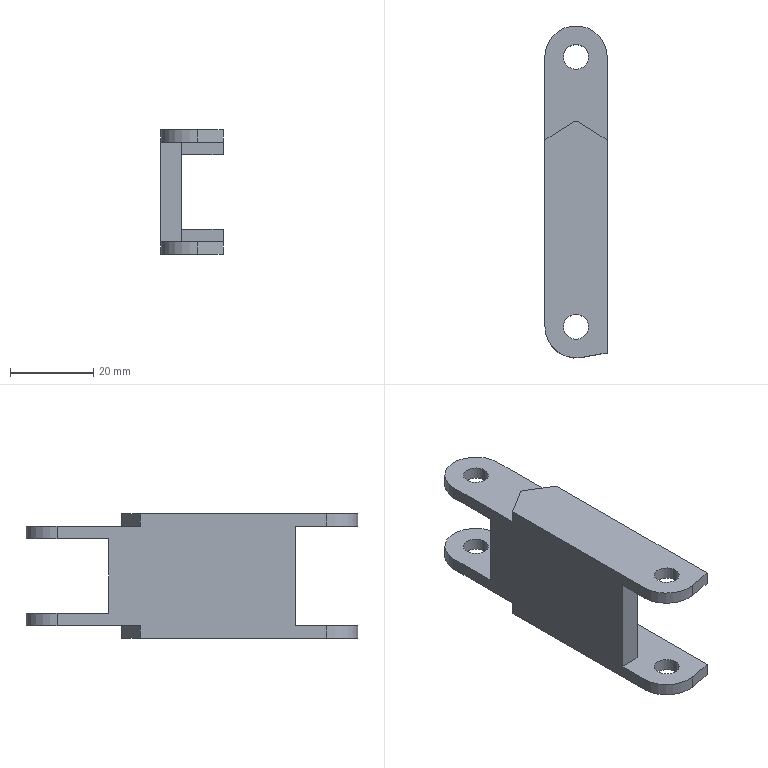Part | SolidWorks | features ICE 4, Extrusion 1, Fillet 1 | 1 solid | 36 faces | box 15 x 80 x 30 mm | volume 12794 mm3 | plane 22 | cylinder 14 | commonest cylinder face diameters 6 x8 15 x4 2 x2
STEP:
#1=CARTESIAN_POINT('',(3.,65.,27.));
#2=VERTEX_POINT('',#1);
#3=CARTESIAN_POINT('',(-3.,65.,27.));
#4=VERTEX_POINT('',#3);
#5=CARTESIAN_POINT('',(0.,65.,27.));
#6=DIRECTION('',(0.,0.,-1.));
#7=DIRECTION('',(-1.,0.,0.));
#8=AXIS2_PLACEMENT_3D('',#5,#6,#7);
#9=CIRCLE('',#8,3.);
#10=EDGE_CURVE('',#2,#4,#9,.T.);
#11=ORIENTED_EDGE('',*,*,#10,.F.);
#12=CARTESIAN_POINT('',(3.,65.,24.));
#13=VERTEX_POINT('',#12);
#14=CARTESIAN_POINT('',(3.,65.,30.));
#15=DIRECTION('',(0.,0.,-1.));
#16=VECTOR('',#15,1000.);
#17=LINE('',#14,#16);
#18=EDGE_CURVE('',#2,#13,#17,.T.);
#19=ORIENTED_EDGE('',*,*,#18,.T.);
#20=CARTESIAN_POINT('',(-3.,65.,24.));
#21=VERTEX_POINT('',#20);
#22=CARTESIAN_POINT('',(0.,65.,24.));
#23=DIRECTION('',(0.,0.,1.));
#24=DIRECTION('',(1.,0.,0.));
#25=AXIS2_PLACEMENT_3D('',#22,#23,#24);
#26=CIRCLE('',#25,3.);
#27=EDGE_CURVE('',#21,#13,#26,.T.);
#28=ORIENTED_EDGE('',*,*,#27,.F.);
#29=CARTESIAN_POINT('',(-3.,65.,30.));
#30=DIRECTION('',(0.,0.,-1.));
#31=VECTOR('',#30,1000.);
#32=LINE('',#29,#31);
#33=EDGE_CURVE('',#4,#21,#32,.T.);
#34=ORIENTED_EDGE('',*,*,#33,.F.);
#35=EDGE_LOOP('',(#11,#19,#28,#34));
#36=FACE_OUTER_BOUND('',#35,.T.);
#37=CARTESIAN_POINT('',(0.,65.,30.));
#38=DIRECTION('',(0.,0.,-1.));
#39=DIRECTION('',(-1.,0.,0.));
#40=AXIS2_PLACEMENT_3D('',#37,#38,#39);
#41=CYLINDRICAL_SURFACE('',#40,3.);
#42=ADVANCED_FACE('',(#36),#41,.F.);
#43=CARTESIAN_POINT('',(-3.,0.,30.));
#44=VERTEX_POINT('',#43);
#45=CARTESIAN_POINT('',(3.,0.,30.));
#46=VERTEX_POINT('',#45);
#47=CARTESIAN_POINT('',(0.,0.,30.));
#48=DIRECTION('',(0.,0.,1.));
#49=DIRECTION('',(1.,0.,0.));
#50=AXIS2_PLACEMENT_3D('',#47,#48,#49);
#51=CIRCLE('',#50,3.);
#52=EDGE_CURVE('',#44,#46,#51,.T.);
#53=ORIENTED_EDGE('',*,*,#52,.T.);
#54=CARTESIAN_POINT('',(3.,0.,27.));
#55=VERTEX_POINT('',#54);
#56=CARTESIAN_POINT('',(3.,0.,30.));
#57=DIRECTION('',(0.,0.,-1.));
#58=VECTOR('',#57,1000.);
#59=LINE('',#56,#58);
#60=EDGE_CURVE('',#46,#55,#59,.T.);
#61=ORIENTED_EDGE('',*,*,#60,.T.);
#62=CARTESIAN_POINT('',(-3.,0.,27.));
#63=VERTEX_POINT('',#62);
#64=CARTESIAN_POINT('',(0.,0.,27.));
#65=DIRECTION('',(0.,0.,1.));
#66=DIRECTION('',(1.,0.,0.));
#67=AXIS2_PLACEMENT_3D('',#64,#65,#66);
#68=CIRCLE('',#67,3.);
#69=EDGE_CURVE('',#63,#55,#68,.T.);
#70=ORIENTED_EDGE('',*,*,#69,.F.);
#71=CARTESIAN_POINT('',(-3.,0.,30.));
#72=DIRECTION('',(0.,0.,-1.));
#73=VECTOR('',#72,1000.);
#74=LINE('',#71,#73);
#75=EDGE_CURVE('',#44,#63,#74,.T.);
#76=ORIENTED_EDGE('',*,*,#75,.F.);
#77=EDGE_LOOP('',(#53,#61,#70,#76));
#78=FACE_OUTER_BOUND('',#77,.T.);
#79=CARTESIAN_POINT('',(0.,0.,30.));
#80=DIRECTION('',(0.,0.,-1.));
#81=DIRECTION('',(-1.,0.,0.));
#82=AXIS2_PLACEMENT_3D('',#79,#80,#81);
#83=CYLINDRICAL_SURFACE('',#82,3.);
#84=ADVANCED_FACE('',(#78),#83,.F.);
#85=CARTESIAN_POINT('',(3.,65.,6.));
#86=VERTEX_POINT('',#85);
#87=CARTESIAN_POINT('',(-3.,65.,6.));
#88=VERTEX_POINT('',#87);
#89=CARTESIAN_POINT('',(0.,65.,6.));
#90=DIRECTION('',(0.,0.,-1.));
#91=DIRECTION('',(-1.,0.,0.));
#92=AXIS2_PLACEMENT_3D('',#89,#90,#91);
#93=CIRCLE('',#92,3.);
#94=EDGE_CURVE('',#86,#88,#93,.T.);
#95=ORIENTED_EDGE('',*,*,#94,.F.);
#96=CARTESIAN_POINT('',(3.,65.,3.));
#97=VERTEX_POINT('',#96);
#98=CARTESIAN_POINT('',(3.,65.,30.));
#99=DIRECTION('',(0.,0.,-1.));
#100=VECTOR('',#99,1000.);
#101=LINE('',#98,#100);
#102=EDGE_CURVE('',#86,#97,#101,.T.);
#103=ORIENTED_EDGE('',*,*,#102,.T.);
#104=CARTESIAN_POINT('',(-3.,65.,3.));
#105=VERTEX_POINT('',#104);
#106=CARTESIAN_POINT('',(0.,65.,3.));
#107=DIRECTION('',(0.,0.,1.));
#108=DIRECTION('',(1.,0.,0.));
#109=AXIS2_PLACEMENT_3D('',#106,#107,#108);
#110=CIRCLE('',#109,3.);
#111=EDGE_CURVE('',#105,#97,#110,.T.);
#112=ORIENTED_EDGE('',*,*,#111,.F.);
#113=CARTESIAN_POINT('',(-3.,65.,30.));
#114=DIRECTION('',(0.,0.,-1.));
#115=VECTOR('',#114,1000.);
#116=LINE('',#113,#115);
#117=EDGE_CURVE('',#88,#105,#116,.T.);
#118=ORIENTED_EDGE('',*,*,#117,.F.);
#119=EDGE_LOOP('',(#95,#103,#112,#118));
#120=FACE_OUTER_BOUND('',#119,.T.);
#121=CARTESIAN_POINT('',(0.,65.,30.));
#122=DIRECTION('',(0.,0.,-1.));
#123=DIRECTION('',(-1.,0.,0.));
#124=AXIS2_PLACEMENT_3D('',#121,#122,#123);
#125=CYLINDRICAL_SURFACE('',#124,3.);
#126=ADVANCED_FACE('',(#120),#125,.F.);
#127=CARTESIAN_POINT('',(3.,0.,3.));
#128=VERTEX_POINT('',#127);
#129=CARTESIAN_POINT('',(-3.,0.,3.));
#130=VERTEX_POINT('',#129);
#131=CARTESIAN_POINT('',(0.,0.,3.));
#132=DIRECTION('',(0.,0.,-1.));
#133=DIRECTION('',(-1.,0.,0.));
#134=AXIS2_PLACEMENT_3D('',#131,#132,#133);
#135=CIRCLE('',#134,3.);
#136=EDGE_CURVE('',#128,#130,#135,.T.);
#137=ORIENTED_EDGE('',*,*,#136,.F.);
#138=CARTESIAN_POINT('',(3.,0.,0.));
#139=VERTEX_POINT('',#138);
#140=CARTESIAN_POINT('',(3.,0.,30.));
#141=DIRECTION('',(0.,0.,-1.));
#142=VECTOR('',#141,1000.);
#143=LINE('',#140,#142);
#144=EDGE_CURVE('',#128,#139,#143,.T.);
#145=ORIENTED_EDGE('',*,*,#144,.T.);
#146=CARTESIAN_POINT('',(-3.,0.,0.));
#147=VERTEX_POINT('',#146);
#148=CARTESIAN_POINT('',(0.,0.,0.));
#149=DIRECTION('',(0.,0.,1.));
#150=DIRECTION('',(1.,0.,0.));
#151=AXIS2_PLACEMENT_3D('',#148,#149,#150);
#152=CIRCLE('',#151,3.);
#153=EDGE_CURVE('',#147,#139,#152,.T.);
#154=ORIENTED_EDGE('',*,*,#153,.F.);
#155=CARTESIAN_POINT('',(-3.,0.,30.));
#156=DIRECTION('',(0.,0.,-1.));
#157=VECTOR('',#156,1000.);
#158=LINE('',#155,#157);
#159=EDGE_CURVE('',#130,#147,#158,.T.);
#160=ORIENTED_EDGE('',*,*,#159,.F.);
#161=EDGE_LOOP('',(#137,#145,#154,#160));
#162=FACE_OUTER_BOUND('',#161,.T.);
#163=CARTESIAN_POINT('',(0.,0.,30.));
#164=DIRECTION('',(0.,0.,-1.));
#165=DIRECTION('',(-1.,0.,0.));
#166=AXIS2_PLACEMENT_3D('',#163,#164,#165);
#167=CYLINDRICAL_SURFACE('',#166,3.);
#168=ADVANCED_FACE('',(#162),#167,.F.);
#169=CARTESIAN_POINT('',(7.5,31.614,6.));
#170=VERTEX_POINT('',#169);
#171=CARTESIAN_POINT('',(7.5,65.,6.));
#172=VERTEX_POINT('',#171);
#173=CARTESIAN_POINT('',(7.5,92.5,6.));
#174=DIRECTION('',(0.,1.,0.));
#175=VECTOR('',#174,1000.);
#176=LINE('',#173,#175);
#177=EDGE_CURVE('',#170,#172,#176,.T.);
#178=ORIENTED_EDGE('',*,*,#177,.F.);
#179=CARTESIAN_POINT('',(7.5,31.614,3.));
#180=VERTEX_POINT('',#179);
#181=CARTESIAN_POINT('',(7.5,31.614,3.));
#182=DIRECTION('',(0.,0.,1.));
#183=VECTOR('',#182,1000.);
#184=LINE('',#181,#183);
#185=EDGE_CURVE('',#180,#170,#184,.T.);
#186=ORIENTED_EDGE('',*,*,#185,.F.);
#187=CARTESIAN_POINT('',(7.5,-6.293,3.));
#188=VERTEX_POINT('',#187);
#189=CARTESIAN_POINT('',(7.5,7.614,3.));
#190=DIRECTION('',(0.,1.,0.));
#191=VECTOR('',#190,1000.);
#192=LINE('',#189,#191);
#193=EDGE_CURVE('',#188,#180,#192,.T.);
#194=ORIENTED_EDGE('',*,*,#193,.F.);
#195=CARTESIAN_POINT('',(7.5,-6.293,0.));
#196=VERTEX_POINT('',#195);
#197=CARTESIAN_POINT('',(7.5,-6.293,30.));
#198=DIRECTION('',(0.,0.,-1.));
#199=VECTOR('',#198,1000.);
#200=LINE('',#197,#199);
#201=EDGE_CURVE('',#188,#196,#200,.T.);
#202=ORIENTED_EDGE('',*,*,#201,.T.);
#203=CARTESIAN_POINT('',(7.5,45.,0.));
#204=VERTEX_POINT('',#203);
#205=CARTESIAN_POINT('',(7.5,65.,0.));
#206=DIRECTION('',(0.,1.,0.));
#207=VECTOR('',#206,1000.);
#208=LINE('',#205,#207);
#209=EDGE_CURVE('',#196,#204,#208,.T.);
#210=ORIENTED_EDGE('',*,*,#209,.T.);
#211=CARTESIAN_POINT('',(7.5,45.,3.));
#212=VERTEX_POINT('',#211);
#213=CARTESIAN_POINT('',(7.5,45.,3.));
#214=DIRECTION('',(0.,0.,-1.));
#215=VECTOR('',#214,1000.);
#216=LINE('',#213,#215);
#217=EDGE_CURVE('',#212,#204,#216,.T.);
#218=ORIENTED_EDGE('',*,*,#217,.F.);
#219=CARTESIAN_POINT('',(7.5,65.,3.));
#220=VERTEX_POINT('',#219);
#221=CARTESIAN_POINT('',(7.5,65.,3.));
#222=DIRECTION('',(0.,1.,0.));
#223=VECTOR('',#222,1000.);
#224=LINE('',#221,#223);
#225=EDGE_CURVE('',#212,#220,#224,.T.);
#226=ORIENTED_EDGE('',*,*,#225,.T.);
#227=CARTESIAN_POINT('',(7.5,65.,30.));
#228=DIRECTION('',(0.,0.,-1.));
#229=VECTOR('',#228,1000.);
#230=LINE('',#227,#229);
#231=EDGE_CURVE('',#172,#220,#230,.T.);
#232=ORIENTED_EDGE('',*,*,#231,.F.);
#233=EDGE_LOOP('',(#178,#186,#194,#202,#210,#218,#226,#232));
#234=FACE_OUTER_BOUND('',#233,.T.);
#235=CARTESIAN_POINT('',(7.5,65.,30.));
#236=DIRECTION('',(-1.,0.,0.));
#237=DIRECTION('',(0.,-1.,0.));
#238=AXIS2_PLACEMENT_3D('',#235,#236,#237);
#239=PLANE('',#238);
#240=ADVANCED_FACE('',(#234),#239,.F.);
#241=ORIENTED_EDGE('',*,*,#153,.T.);
#242=CARTESIAN_POINT('',(0.,0.,0.));
#243=DIRECTION('',(0.,0.,1.));
#244=DIRECTION('',(1.,0.,0.));
#245=AXIS2_PLACEMENT_3D('',#242,#243,#244);
#246=CIRCLE('',#245,3.);
#247=EDGE_CURVE('',#139,#147,#246,.T.);
#248=ORIENTED_EDGE('',*,*,#247,.T.);
#249=EDGE_LOOP('',(#241,#248));
#250=FACE_BOUND('',#249,.T.);
#251=CARTESIAN_POINT('',(-7.5,45.,0.));
#252=VERTEX_POINT('',#251);
#253=CARTESIAN_POINT('',(-0.5299,49.355,0.));
#254=VERTEX_POINT('',#253);
#255=CARTESIAN_POINT('',(6.882,53.987,0.));
#256=DIRECTION('',(0.848,0.5299,0.));
#257=VECTOR('',#256,1000.);
#258=LINE('',#255,#257);
#259=EDGE_CURVE('',#252,#254,#258,.T.);
#260=ORIENTED_EDGE('',*,*,#259,.T.);
#261=CARTESIAN_POINT('',(0.5299,49.355,0.));
#262=VERTEX_POINT('',#261);
#263=CARTESIAN_POINT('',(0.,48.507,0.));
#264=DIRECTION('',(0.,0.,-1.));
#265=DIRECTION('',(1.,0.,0.));
#266=AXIS2_PLACEMENT_3D('',#263,#264,#265);
#267=CIRCLE('',#266,1.);
#268=EDGE_CURVE('',#254,#262,#267,.T.);
#269=ORIENTED_EDGE('',*,*,#268,.T.);
#270=CARTESIAN_POINT('',(-6.882,53.987,0.));
#271=DIRECTION('',(0.848,-0.5299,0.));
#272=VECTOR('',#271,1000.);
#273=LINE('',#270,#272);
#274=EDGE_CURVE('',#262,#204,#273,.T.);
#275=ORIENTED_EDGE('',*,*,#274,.T.);
#276=ORIENTED_EDGE('',*,*,#209,.F.);
#277=CARTESIAN_POINT('',(1.302,-7.386,0.));
#278=VERTEX_POINT('',#277);
#279=CARTESIAN_POINT('',(7.5,-6.293,0.));
#280=DIRECTION('',(0.9848,0.1736,0.));
#281=VECTOR('',#280,1000.);
#282=LINE('',#279,#281);
#283=EDGE_CURVE('',#278,#196,#282,.T.);
#284=ORIENTED_EDGE('',*,*,#283,.F.);
#285=CARTESIAN_POINT('',(-7.5,0.,0.));
#286=VERTEX_POINT('',#285);
#287=CARTESIAN_POINT('',(0.,0.,0.));
#288=DIRECTION('',(0.,0.,1.));
#289=DIRECTION('',(1.,0.,0.));
#290=AXIS2_PLACEMENT_3D('',#287,#288,#289);
#291=CIRCLE('',#290,7.5);
#292=EDGE_CURVE('',#286,#278,#291,.T.);
#293=ORIENTED_EDGE('',*,*,#292,.F.);
#294=CARTESIAN_POINT('',(-7.5,65.,0.));
#295=DIRECTION('',(0.,-1.,0.));
#296=VECTOR('',#295,1000.);
#297=LINE('',#294,#296);
#298=EDGE_CURVE('',#252,#286,#297,.T.);
#299=ORIENTED_EDGE('',*,*,#298,.F.);
#300=EDGE_LOOP('',(#260,#269,#275,#276,#284,#293,#299));
#301=FACE_OUTER_BOUND('',#300,.T.);
#302=CARTESIAN_POINT('',(0.,65.,0.));
#303=DIRECTION('',(0.,0.,1.));
#304=DIRECTION('',(1.,0.,0.));
#305=AXIS2_PLACEMENT_3D('',#302,#303,#304);
#306=PLANE('',#305);
#307=ADVANCED_FACE('',(#250,#301),#306,.F.);
#308=CARTESIAN_POINT('',(-7.5,45.,3.));
#309=VERTEX_POINT('',#308);
#310=CARTESIAN_POINT('',(-7.5,45.,3.));
#311=DIRECTION('',(0.,0.,-1.));
#312=VECTOR('',#311,1000.);
#313=LINE('',#310,#312);
#314=EDGE_CURVE('',#309,#252,#313,.T.);
#315=ORIENTED_EDGE('',*,*,#314,.T.);
#316=ORIENTED_EDGE('',*,*,#298,.T.);
#317=CARTESIAN_POINT('',(-7.5,0.,3.));
#318=VERTEX_POINT('',#317);
#319=CARTESIAN_POINT('',(-7.5,0.,30.));
#320=DIRECTION('',(0.,0.,-1.));
#321=VECTOR('',#320,1000.);
#322=LINE('',#319,#321);
#323=EDGE_CURVE('',#318,#286,#322,.T.);
#324=ORIENTED_EDGE('',*,*,#323,.F.);
#325=CARTESIAN_POINT('',(-7.5,7.614,3.));
#326=VERTEX_POINT('',#325);
#327=CARTESIAN_POINT('',(-7.5,65.,3.));
#328=DIRECTION('',(0.,1.,0.));
#329=VECTOR('',#328,1000.);
#330=LINE('',#327,#329);
#331=EDGE_CURVE('',#318,#326,#330,.T.);
#332=ORIENTED_EDGE('',*,*,#331,.T.);
#333=CARTESIAN_POINT('',(-7.5,7.614,27.));
#334=VERTEX_POINT('',#333);
#335=CARTESIAN_POINT('',(-7.5,7.614,30.));
#336=DIRECTION('',(0.,0.,1.));
#337=VECTOR('',#336,1000.);
#338=LINE('',#335,#337);
#339=EDGE_CURVE('',#326,#334,#338,.T.);
#340=ORIENTED_EDGE('',*,*,#339,.T.);
#341=CARTESIAN_POINT('',(-7.5,0.,27.));
#342=VERTEX_POINT('',#341);
#343=CARTESIAN_POINT('',(-7.5,65.,27.));
#344=DIRECTION('',(0.,-1.,0.));
#345=VECTOR('',#344,1000.);
#346=LINE('',#343,#345);
#347=EDGE_CURVE('',#334,#342,#346,.T.);
#348=ORIENTED_EDGE('',*,*,#347,.T.);
#349=CARTESIAN_POINT('',(-7.5,0.,30.));
#350=VERTEX_POINT('',#349);
#351=CARTESIAN_POINT('',(-7.5,0.,30.));
#352=DIRECTION('',(0.,0.,-1.));
#353=VECTOR('',#352,1000.);
#354=LINE('',#351,#353);
#355=EDGE_CURVE('',#350,#342,#354,.T.);
#356=ORIENTED_EDGE('',*,*,#355,.F.);
#357=CARTESIAN_POINT('',(-7.5,45.,30.));
#358=VERTEX_POINT('',#357);
#359=CARTESIAN_POINT('',(-7.5,65.,30.));
#360=DIRECTION('',(0.,-1.,0.));
#361=VECTOR('',#360,1000.);
#362=LINE('',#359,#361);
#363=EDGE_CURVE('',#358,#350,#362,.T.);
#364=ORIENTED_EDGE('',*,*,#363,.F.);
#365=CARTESIAN_POINT('',(-7.5,45.,27.));
#366=VERTEX_POINT('',#365);
#367=CARTESIAN_POINT('',(-7.5,45.,27.));
#368=DIRECTION('',(0.,0.,1.));
#369=VECTOR('',#368,1000.);
#370=LINE('',#367,#369);
#371=EDGE_CURVE('',#366,#358,#370,.T.);
#372=ORIENTED_EDGE('',*,*,#371,.F.);
#373=CARTESIAN_POINT('',(-7.5,65.,27.));
#374=VERTEX_POINT('',#373);
#375=CARTESIAN_POINT('',(-7.5,65.,27.));
#376=DIRECTION('',(0.,1.,0.));
#377=VECTOR('',#376,1000.);
#378=LINE('',#375,#377);
#379=EDGE_CURVE('',#366,#374,#378,.T.);
#380=ORIENTED_EDGE('',*,*,#379,.T.);
#381=CARTESIAN_POINT('',(-7.5,65.,24.));
#382=VERTEX_POINT('',#381);
#383=CARTESIAN_POINT('',(-7.5,65.,30.));
#384=DIRECTION('',(0.,0.,-1.));
#385=VECTOR('',#384,1000.);
#386=LINE('',#383,#385);
#387=EDGE_CURVE('',#374,#382,#386,.T.);
#388=ORIENTED_EDGE('',*,*,#387,.T.);
#389=CARTESIAN_POINT('',(-7.5,52.5,24.));
#390=VERTEX_POINT('',#389);
#391=CARTESIAN_POINT('',(-7.5,65.,24.));
#392=DIRECTION('',(0.,-1.,0.));
#393=VECTOR('',#392,1000.);
#394=LINE('',#391,#393);
#395=EDGE_CURVE('',#382,#390,#394,.T.);
#396=ORIENTED_EDGE('',*,*,#395,.T.);
#397=CARTESIAN_POINT('',(-7.5,52.5,6.));
#398=VERTEX_POINT('',#397);
#399=CARTESIAN_POINT('',(-7.5,52.5,30.));
#400=DIRECTION('',(0.,0.,-1.));
#401=VECTOR('',#400,1000.);
#402=LINE('',#399,#401);
#403=EDGE_CURVE('',#390,#398,#402,.T.);
#404=ORIENTED_EDGE('',*,*,#403,.T.);
#405=CARTESIAN_POINT('',(-7.5,65.,6.));
#406=VERTEX_POINT('',#405);
#407=CARTESIAN_POINT('',(-7.5,65.,6.));
#408=DIRECTION('',(0.,1.,0.));
#409=VECTOR('',#408,1000.);
#410=LINE('',#407,#409);
#411=EDGE_CURVE('',#398,#406,#410,.T.);
#412=ORIENTED_EDGE('',*,*,#411,.T.);
#413=CARTESIAN_POINT('',(-7.5,65.,3.));
#414=VERTEX_POINT('',#413);
#415=CARTESIAN_POINT('',(-7.5,65.,30.));
#416=DIRECTION('',(0.,0.,-1.));
#417=VECTOR('',#416,1000.);
#418=LINE('',#415,#417);
#419=EDGE_CURVE('',#406,#414,#418,.T.);
#420=ORIENTED_EDGE('',*,*,#419,.T.);
#421=CARTESIAN_POINT('',(-7.5,65.,3.));
#422=DIRECTION('',(0.,-1.,0.));
#423=VECTOR('',#422,1000.);
#424=LINE('',#421,#423);
#425=EDGE_CURVE('',#414,#309,#424,.T.);
#426=ORIENTED_EDGE('',*,*,#425,.T.);
#427=EDGE_LOOP('',(#315,#316,#324,#332,#340,#348,#356,#364,#372,#380,#388,#396,#404,#412,#420,#426));
#428=FACE_OUTER_BOUND('',#427,.T.);
#429=CARTESIAN_POINT('',(-7.5,65.,30.));
#430=DIRECTION('',(1.,0.,0.));
#431=DIRECTION('',(0.,0.,-1.));
#432=AXIS2_PLACEMENT_3D('',#429,#430,#431);
#433=PLANE('',#432);
#434=ADVANCED_FACE('',(#428),#433,.F.);
#435=CARTESIAN_POINT('',(7.5,31.614,24.));
#436=VERTEX_POINT('',#435);
#437=CARTESIAN_POINT('',(7.5,31.614,27.));
#438=VERTEX_POINT('',#437);
#439=CARTESIAN_POINT('',(7.5,31.614,24.));
#440=DIRECTION('',(0.,0.,1.));
#441=VECTOR('',#440,1000.);
#442=LINE('',#439,#441);
#443=EDGE_CURVE('',#436,#438,#442,.T.);
#444=ORIENTED_EDGE('',*,*,#443,.F.);
#445=CARTESIAN_POINT('',(7.5,65.,24.));
#446=VERTEX_POINT('',#445);
#447=CARTESIAN_POINT('',(7.5,92.5,24.));
#448=DIRECTION('',(0.,-1.,0.));
#449=VECTOR('',#448,1000.);
#450=LINE('',#447,#449);
#451=EDGE_CURVE('',#446,#436,#450,.T.);
#452=ORIENTED_EDGE('',*,*,#451,.F.);
#453=CARTESIAN_POINT('',(7.5,65.,27.));
#454=VERTEX_POINT('',#453);
#455=CARTESIAN_POINT('',(7.5,65.,30.));
#456=DIRECTION('',(0.,0.,-1.));
#457=VECTOR('',#456,1000.);
#458=LINE('',#455,#457);
#459=EDGE_CURVE('',#454,#446,#458,.T.);
#460=ORIENTED_EDGE('',*,*,#459,.F.);
#461=CARTESIAN_POINT('',(7.5,45.,27.));
#462=VERTEX_POINT('',#461);
#463=CARTESIAN_POINT('',(7.5,65.,27.));
#464=DIRECTION('',(0.,-1.,0.));
#465=VECTOR('',#464,1000.);
#466=LINE('',#463,#465);
#467=EDGE_CURVE('',#454,#462,#466,.T.);
#468=ORIENTED_EDGE('',*,*,#467,.T.);
#469=CARTESIAN_POINT('',(7.5,45.,30.));
#470=VERTEX_POINT('',#469);
#471=CARTESIAN_POINT('',(7.5,45.,27.));
#472=DIRECTION('',(0.,0.,1.));
#473=VECTOR('',#472,1000.);
#474=LINE('',#471,#473);
#475=EDGE_CURVE('',#462,#470,#474,.T.);
#476=ORIENTED_EDGE('',*,*,#475,.T.);
#477=CARTESIAN_POINT('',(7.5,-6.293,30.));
#478=VERTEX_POINT('',#477);
#479=CARTESIAN_POINT('',(7.5,65.,30.));
#480=DIRECTION('',(0.,1.,0.));
#481=VECTOR('',#480,1000.);
#482=LINE('',#479,#481);
#483=EDGE_CURVE('',#478,#470,#482,.T.);
#484=ORIENTED_EDGE('',*,*,#483,.F.);
#485=CARTESIAN_POINT('',(7.5,-6.293,27.));
#486=VERTEX_POINT('',#485);
#487=CARTESIAN_POINT('',(7.5,-6.293,30.));
#488=DIRECTION('',(0.,0.,-1.));
#489=VECTOR('',#488,1000.);
#490=LINE('',#487,#489);
#491=EDGE_CURVE('',#478,#486,#490,.T.);
#492=ORIENTED_EDGE('',*,*,#491,.T.);
#493=CARTESIAN_POINT('',(7.5,7.614,27.));
#494=DIRECTION('',(0.,-1.,0.));
#495=VECTOR('',#494,1000.);
#496=LINE('',#493,#495);
#497=EDGE_CURVE('',#438,#486,#496,.T.);
#498=ORIENTED_EDGE('',*,*,#497,.F.);
#499=EDGE_LOOP('',(#444,#452,#460,#468,#476,#484,#492,#498));
#500=FACE_OUTER_BOUND('',#499,.T.);
#501=CARTESIAN_POINT('',(7.5,65.,30.));
#502=DIRECTION('',(-1.,0.,0.));
#503=DIRECTION('',(0.,-1.,0.));
#504=AXIS2_PLACEMENT_3D('',#501,#502,#503);
#505=PLANE('',#504);
#506=ADVANCED_FACE('',(#500),#505,.F.);
#507=ORIENTED_EDGE('',*,*,#231,.T.);
#508=CARTESIAN_POINT('',(0.,65.,3.));
#509=DIRECTION('',(0.,0.,1.));
#510=DIRECTION('',(1.,0.,0.));
#511=AXIS2_PLACEMENT_3D('',#508,#509,#510);
#512=CIRCLE('',#511,7.5);
#513=EDGE_CURVE('',#220,#414,#512,.T.);
#514=ORIENTED_EDGE('',*,*,#513,.T.);
#515=ORIENTED_EDGE('',*,*,#419,.F.);
#516=CARTESIAN_POINT('',(0.,65.,6.));
#517=DIRECTION('',(0.,0.,-1.));
#518=DIRECTION('',(-1.,0.,0.));
#519=AXIS2_PLACEMENT_3D('',#516,#517,#518);
#520=CIRCLE('',#519,7.5);
#521=EDGE_CURVE('',#406,#172,#520,.T.);
#522=ORIENTED_EDGE('',*,*,#521,.T.);
#523=EDGE_LOOP('',(#507,#514,#515,#522));
#524=FACE_OUTER_BOUND('',#523,.T.);
#525=CARTESIAN_POINT('',(0.,65.,30.));
#526=DIRECTION('',(0.,0.,-1.));
#527=DIRECTION('',(-1.,0.,0.));
#528=AXIS2_PLACEMENT_3D('',#525,#526,#527);
#529=CYLINDRICAL_SURFACE('',#528,7.5);
#530=ADVANCED_FACE('',(#524),#529,.T.);
#531=CARTESIAN_POINT('',(1.302,-7.386,3.));
#532=VERTEX_POINT('',#531);
#533=CARTESIAN_POINT('',(1.302,-7.386,30.));
#534=DIRECTION('',(0.,0.,-1.));
#535=VECTOR('',#534,1000.);
#536=LINE('',#533,#535);
#537=EDGE_CURVE('',#532,#278,#536,.T.);
#538=ORIENTED_EDGE('',*,*,#537,.F.);
#539=CARTESIAN_POINT('',(0.,0.,3.));
#540=DIRECTION('',(0.,0.,-1.));
#541=DIRECTION('',(-1.,0.,0.));
#542=AXIS2_PLACEMENT_3D('',#539,#540,#541);
#543=CIRCLE('',#542,7.5);
#544=EDGE_CURVE('',#532,#318,#543,.T.);
#545=ORIENTED_EDGE('',*,*,#544,.T.);
#546=ORIENTED_EDGE('',*,*,#323,.T.);
#547=ORIENTED_EDGE('',*,*,#292,.T.);
#548=EDGE_LOOP('',(#538,#545,#546,#547));
#549=FACE_OUTER_BOUND('',#548,.T.);
#550=CARTESIAN_POINT('',(0.,0.,30.));
#551=DIRECTION('',(0.,0.,-1.));
#552=DIRECTION('',(-1.,0.,0.));
#553=AXIS2_PLACEMENT_3D('',#550,#551,#552);
#554=CYLINDRICAL_SURFACE('',#553,7.5);
#555=ADVANCED_FACE('',(#549),#554,.T.);
#556=ORIENTED_EDGE('',*,*,#201,.F.);
#557=CARTESIAN_POINT('',(7.5,-6.293,3.));
#558=DIRECTION('',(-0.9848,-0.1736,0.));
#559=VECTOR('',#558,1000.);
#560=LINE('',#557,#559);
#561=EDGE_CURVE('',#188,#532,#560,.T.);
#562=ORIENTED_EDGE('',*,*,#561,.T.);
#563=ORIENTED_EDGE('',*,*,#537,.T.);
#564=ORIENTED_EDGE('',*,*,#283,.T.);
#565=EDGE_LOOP('',(#556,#562,#563,#564));
#566=FACE_OUTER_BOUND('',#565,.T.);
#567=CARTESIAN_POINT('',(7.5,-6.293,30.));
#568=DIRECTION('',(-0.1736,0.9848,0.));
#569=DIRECTION('',(-0.9848,-0.1736,0.));
#570=AXIS2_PLACEMENT_3D('',#567,#568,#569);
#571=PLANE('',#570);
#572=ADVANCED_FACE('',(#566),#571,.F.);
#573=ORIENTED_EDGE('',*,*,#144,.F.);
#574=CARTESIAN_POINT('',(0.,0.,3.));
#575=DIRECTION('',(0.,0.,-1.));
#576=DIRECTION('',(-1.,0.,0.));
#577=AXIS2_PLACEMENT_3D('',#574,#575,#576);
#578=CIRCLE('',#577,3.);
#579=EDGE_CURVE('',#130,#128,#578,.T.);
#580=ORIENTED_EDGE('',*,*,#579,.F.);
#581=ORIENTED_EDGE('',*,*,#159,.T.);
#582=ORIENTED_EDGE('',*,*,#247,.F.);
#583=EDGE_LOOP('',(#573,#580,#581,#582));
#584=FACE_OUTER_BOUND('',#583,.T.);
#585=CARTESIAN_POINT('',(0.,0.,30.));
#586=DIRECTION('',(0.,0.,-1.));
#587=DIRECTION('',(-1.,0.,0.));
#588=AXIS2_PLACEMENT_3D('',#585,#586,#587);
#589=CYLINDRICAL_SURFACE('',#588,3.);
#590=ADVANCED_FACE('',(#584),#589,.F.);
#591=ORIENTED_EDGE('',*,*,#102,.F.);
#592=CARTESIAN_POINT('',(0.,65.,6.));
#593=DIRECTION('',(0.,0.,-1.));
#594=DIRECTION('',(-1.,0.,0.));
#595=AXIS2_PLACEMENT_3D('',#592,#593,#594);
#596=CIRCLE('',#595,3.);
#597=EDGE_CURVE('',#88,#86,#596,.T.);
#598=ORIENTED_EDGE('',*,*,#597,.F.);
#599=ORIENTED_EDGE('',*,*,#117,.T.);
#600=CARTESIAN_POINT('',(0.,65.,3.));
#601=DIRECTION('',(0.,0.,1.));
#602=DIRECTION('',(1.,0.,0.));
#603=AXIS2_PLACEMENT_3D('',#600,#601,#602);
#604=CIRCLE('',#603,3.);
#605=EDGE_CURVE('',#97,#105,#604,.T.);
#606=ORIENTED_EDGE('',*,*,#605,.F.);
#607=EDGE_LOOP('',(#591,#598,#599,#606));
#608=FACE_OUTER_BOUND('',#607,.T.);
#609=CARTESIAN_POINT('',(0.,65.,30.));
#610=DIRECTION('',(0.,0.,-1.));
#611=DIRECTION('',(-1.,0.,0.));
#612=AXIS2_PLACEMENT_3D('',#609,#610,#611);
#613=CYLINDRICAL_SURFACE('',#612,3.);
#614=ADVANCED_FACE('',(#608),#613,.F.);
#615=CARTESIAN_POINT('',(0.5299,49.355,30.));
#616=VERTEX_POINT('',#615);
#617=CARTESIAN_POINT('',(0.,49.687,30.));
#618=DIRECTION('',(0.848,-0.5299,0.));
#619=VECTOR('',#618,1000.);
#620=LINE('',#617,#619);
#621=EDGE_CURVE('',#616,#470,#620,.T.);
#622=ORIENTED_EDGE('',*,*,#621,.F.);
#623=CARTESIAN_POINT('',(-0.5299,49.355,30.));
#624=VERTEX_POINT('',#623);
#625=CARTESIAN_POINT('',(0.,48.507,30.));
#626=DIRECTION('',(0.,0.,1.));
#627=DIRECTION('',(1.,0.,0.));
#628=AXIS2_PLACEMENT_3D('',#625,#626,#627);
#629=CIRCLE('',#628,1.);
#630=EDGE_CURVE('',#616,#624,#629,.T.);
#631=ORIENTED_EDGE('',*,*,#630,.T.);
#632=CARTESIAN_POINT('',(-7.5,45.,30.));
#633=DIRECTION('',(0.848,0.5299,0.));
#634=VECTOR('',#633,1000.);
#635=LINE('',#632,#634);
#636=EDGE_CURVE('',#358,#624,#635,.T.);
#637=ORIENTED_EDGE('',*,*,#636,.F.);
#638=ORIENTED_EDGE('',*,*,#363,.T.);
#639=CARTESIAN_POINT('',(1.302,-7.386,30.));
#640=VERTEX_POINT('',#639);
#641=CARTESIAN_POINT('',(0.,0.,30.));
#642=DIRECTION('',(0.,0.,1.));
#643=DIRECTION('',(1.,0.,0.));
#644=AXIS2_PLACEMENT_3D('',#641,#642,#643);
#645=CIRCLE('',#644,7.5);
#646=EDGE_CURVE('',#350,#640,#645,.T.);
#647=ORIENTED_EDGE('',*,*,#646,.T.);
#648=CARTESIAN_POINT('',(7.5,-6.293,30.));
#649=DIRECTION('',(0.9848,0.1736,0.));
#650=VECTOR('',#649,1000.);
#651=LINE('',#648,#650);
#652=EDGE_CURVE('',#640,#478,#651,.T.);
#653=ORIENTED_EDGE('',*,*,#652,.T.);
#654=ORIENTED_EDGE('',*,*,#483,.T.);
#655=EDGE_LOOP('',(#622,#631,#637,#638,#647,#653,#654));
#656=FACE_OUTER_BOUND('',#655,.T.);
#657=ORIENTED_EDGE('',*,*,#52,.F.);
#658=CARTESIAN_POINT('',(0.,0.,30.));
#659=DIRECTION('',(0.,0.,1.));
#660=DIRECTION('',(1.,0.,0.));
#661=AXIS2_PLACEMENT_3D('',#658,#659,#660);
#662=CIRCLE('',#661,3.);
#663=EDGE_CURVE('',#46,#44,#662,.T.);
#664=ORIENTED_EDGE('',*,*,#663,.F.);
#665=EDGE_LOOP('',(#657,#664));
#666=FACE_BOUND('',#665,.T.);
#667=CARTESIAN_POINT('',(0.,65.,30.));
#668=DIRECTION('',(0.,0.,1.));
#669=DIRECTION('',(1.,0.,0.));
#670=AXIS2_PLACEMENT_3D('',#667,#668,#669);
#671=PLANE('',#670);
#672=ADVANCED_FACE('',(#656,#666),#671,.T.);
#673=ORIENTED_EDGE('',*,*,#387,.F.);
#674=CARTESIAN_POINT('',(0.,65.,27.));
#675=DIRECTION('',(0.,0.,-1.));
#676=DIRECTION('',(-1.,0.,0.));
#677=AXIS2_PLACEMENT_3D('',#674,#675,#676);
#678=CIRCLE('',#677,7.5);
#679=EDGE_CURVE('',#374,#454,#678,.T.);
#680=ORIENTED_EDGE('',*,*,#679,.T.);
#681=ORIENTED_EDGE('',*,*,#459,.T.);
#682=CARTESIAN_POINT('',(0.,65.,24.));
#683=DIRECTION('',(0.,0.,1.));
#684=DIRECTION('',(1.,0.,0.));
#685=AXIS2_PLACEMENT_3D('',#682,#683,#684);
#686=CIRCLE('',#685,7.5);
#687=EDGE_CURVE('',#446,#382,#686,.T.);
#688=ORIENTED_EDGE('',*,*,#687,.T.);
#689=EDGE_LOOP('',(#673,#680,#681,#688));
#690=FACE_OUTER_BOUND('',#689,.T.);
#691=CARTESIAN_POINT('',(0.,65.,30.));
#692=DIRECTION('',(0.,0.,-1.));
#693=DIRECTION('',(-1.,0.,0.));
#694=AXIS2_PLACEMENT_3D('',#691,#692,#693);
#695=CYLINDRICAL_SURFACE('',#694,7.5);
#696=ADVANCED_FACE('',(#690),#695,.T.);
#697=ORIENTED_EDGE('',*,*,#355,.T.);
#698=CARTESIAN_POINT('',(1.302,-7.386,27.));
#699=VERTEX_POINT('',#698);
#700=CARTESIAN_POINT('',(0.,0.,27.));
#701=DIRECTION('',(0.,0.,1.));
#702=DIRECTION('',(1.,0.,0.));
#703=AXIS2_PLACEMENT_3D('',#700,#701,#702);
#704=CIRCLE('',#703,7.5);
#705=EDGE_CURVE('',#342,#699,#704,.T.);
#706=ORIENTED_EDGE('',*,*,#705,.T.);
#707=CARTESIAN_POINT('',(1.302,-7.386,30.));
#708=DIRECTION('',(0.,0.,-1.));
#709=VECTOR('',#708,1000.);
#710=LINE('',#707,#709);
#711=EDGE_CURVE('',#640,#699,#710,.T.);
#712=ORIENTED_EDGE('',*,*,#711,.F.);
#713=ORIENTED_EDGE('',*,*,#646,.F.);
#714=EDGE_LOOP('',(#697,#706,#712,#713));
#715=FACE_OUTER_BOUND('',#714,.T.);
#716=CARTESIAN_POINT('',(0.,0.,30.));
#717=DIRECTION('',(0.,0.,-1.));
#718=DIRECTION('',(-1.,0.,0.));
#719=AXIS2_PLACEMENT_3D('',#716,#717,#718);
#720=CYLINDRICAL_SURFACE('',#719,7.5);
#721=ADVANCED_FACE('',(#715),#720,.T.);
#722=ORIENTED_EDGE('',*,*,#711,.T.);
#723=CARTESIAN_POINT('',(7.5,-6.293,27.));
#724=DIRECTION('',(0.9848,0.1736,0.));
#725=VECTOR('',#724,1000.);
#726=LINE('',#723,#725);
#727=EDGE_CURVE('',#699,#486,#726,.T.);
#728=ORIENTED_EDGE('',*,*,#727,.T.);
#729=ORIENTED_EDGE('',*,*,#491,.F.);
#730=ORIENTED_EDGE('',*,*,#652,.F.);
#731=EDGE_LOOP('',(#722,#728,#729,#730));
#732=FACE_OUTER_BOUND('',#731,.T.);
#733=CARTESIAN_POINT('',(7.5,-6.293,30.));
#734=DIRECTION('',(-0.1736,0.9848,0.));
#735=DIRECTION('',(-0.9848,-0.1736,0.));
#736=AXIS2_PLACEMENT_3D('',#733,#734,#735);
#737=PLANE('',#736);
#738=ADVANCED_FACE('',(#732),#737,.F.);
#739=ORIENTED_EDGE('',*,*,#60,.F.);
#740=ORIENTED_EDGE('',*,*,#663,.T.);
#741=ORIENTED_EDGE('',*,*,#75,.T.);
#742=CARTESIAN_POINT('',(0.,0.,27.));
#743=DIRECTION('',(0.,0.,1.));
#744=DIRECTION('',(1.,0.,0.));
#745=AXIS2_PLACEMENT_3D('',#742,#743,#744);
#746=CIRCLE('',#745,3.);
#747=EDGE_CURVE('',#55,#63,#746,.T.);
#748=ORIENTED_EDGE('',*,*,#747,.F.);
#749=EDGE_LOOP('',(#739,#740,#741,#748));
#750=FACE_OUTER_BOUND('',#749,.T.);
#751=CARTESIAN_POINT('',(0.,0.,30.));
#752=DIRECTION('',(0.,0.,-1.));
#753=DIRECTION('',(-1.,0.,0.));
#754=AXIS2_PLACEMENT_3D('',#751,#752,#753);
#755=CYLINDRICAL_SURFACE('',#754,3.);
#756=ADVANCED_FACE('',(#750),#755,.F.);
#757=ORIENTED_EDGE('',*,*,#18,.F.);
#758=CARTESIAN_POINT('',(0.,65.,27.));
#759=DIRECTION('',(0.,0.,-1.));
#760=DIRECTION('',(-1.,0.,0.));
#761=AXIS2_PLACEMENT_3D('',#758,#759,#760);
#762=CIRCLE('',#761,3.);
#763=EDGE_CURVE('',#4,#2,#762,.T.);
#764=ORIENTED_EDGE('',*,*,#763,.F.);
#765=ORIENTED_EDGE('',*,*,#33,.T.);
#766=CARTESIAN_POINT('',(0.,65.,24.));
#767=DIRECTION('',(0.,0.,1.));
#768=DIRECTION('',(1.,0.,0.));
#769=AXIS2_PLACEMENT_3D('',#766,#767,#768);
#770=CIRCLE('',#769,3.);
#771=EDGE_CURVE('',#13,#21,#770,.T.);
#772=ORIENTED_EDGE('',*,*,#771,.F.);
#773=EDGE_LOOP('',(#757,#764,#765,#772));
#774=FACE_OUTER_BOUND('',#773,.T.);
#775=CARTESIAN_POINT('',(0.,65.,30.));
#776=DIRECTION('',(0.,0.,-1.));
#777=DIRECTION('',(-1.,0.,0.));
#778=AXIS2_PLACEMENT_3D('',#775,#776,#777);
#779=CYLINDRICAL_SURFACE('',#778,3.);
#780=ADVANCED_FACE('',(#774),#779,.F.);
#781=CARTESIAN_POINT('',(-2.5,52.5,24.));
#782=VERTEX_POINT('',#781);
#783=CARTESIAN_POINT('',(-34.5,52.5,24.));
#784=DIRECTION('',(1.,0.,0.));
#785=VECTOR('',#784,1000.);
#786=LINE('',#783,#785);
#787=EDGE_CURVE('',#390,#782,#786,.T.);
#788=ORIENTED_EDGE('',*,*,#787,.T.);
#789=CARTESIAN_POINT('',(-2.5,52.5,6.));
#790=VERTEX_POINT('',#789);
#791=CARTESIAN_POINT('',(-2.5,52.5,24.));
#792=DIRECTION('',(0.,0.,-1.));
#793=VECTOR('',#792,1000.);
#794=LINE('',#791,#793);
#795=EDGE_CURVE('',#782,#790,#794,.T.);
#796=ORIENTED_EDGE('',*,*,#795,.T.);
#797=CARTESIAN_POINT('',(-34.5,52.5,6.));
#798=DIRECTION('',(1.,0.,0.));
#799=VECTOR('',#798,1000.);
#800=LINE('',#797,#799);
#801=EDGE_CURVE('',#398,#790,#800,.T.);
#802=ORIENTED_EDGE('',*,*,#801,.F.);
#803=ORIENTED_EDGE('',*,*,#403,.F.);
#804=EDGE_LOOP('',(#788,#796,#802,#803));
#805=FACE_OUTER_BOUND('',#804,.T.);
#806=CARTESIAN_POINT('',(-34.5,52.5,24.));
#807=DIRECTION('',(0.,-1.,0.));
#808=DIRECTION('',(1.,0.,0.));
#809=AXIS2_PLACEMENT_3D('',#806,#807,#808);
#810=PLANE('',#809);
#811=ADVANCED_FACE('',(#805),#810,.F.);
#812=ORIENTED_EDGE('',*,*,#597,.T.);
#813=ORIENTED_EDGE('',*,*,#94,.T.);
#814=EDGE_LOOP('',(#812,#813));
#815=FACE_BOUND('',#814,.T.);
#816=ORIENTED_EDGE('',*,*,#801,.T.);
#817=CARTESIAN_POINT('',(-2.5,31.614,6.));
#818=VERTEX_POINT('',#817);
#819=CARTESIAN_POINT('',(-2.5,73.386,6.));
#820=DIRECTION('',(0.,1.,0.));
#821=VECTOR('',#820,1000.);
#822=LINE('',#819,#821);
#823=EDGE_CURVE('',#818,#790,#822,.T.);
#824=ORIENTED_EDGE('',*,*,#823,.F.);
#825=CARTESIAN_POINT('',(-2.5,31.614,6.));
#826=DIRECTION('',(1.,0.,0.));
#827=VECTOR('',#826,1000.);
#828=LINE('',#825,#827);
#829=EDGE_CURVE('',#818,#170,#828,.T.);
#830=ORIENTED_EDGE('',*,*,#829,.T.);
#831=ORIENTED_EDGE('',*,*,#177,.T.);
#832=ORIENTED_EDGE('',*,*,#521,.F.);
#833=ORIENTED_EDGE('',*,*,#411,.F.);
#834=EDGE_LOOP('',(#816,#824,#830,#831,#832,#833));
#835=FACE_OUTER_BOUND('',#834,.T.);
#836=CARTESIAN_POINT('',(-34.5,92.5,6.));
#837=DIRECTION('',(0.,0.,-1.));
#838=DIRECTION('',(-1.,0.,0.));
#839=AXIS2_PLACEMENT_3D('',#836,#837,#838);
#840=PLANE('',#839);
#841=ADVANCED_FACE('',(#815,#835),#840,.F.);
#842=ORIENTED_EDGE('',*,*,#27,.T.);
#843=ORIENTED_EDGE('',*,*,#771,.T.);
#844=EDGE_LOOP('',(#842,#843));
#845=FACE_BOUND('',#844,.T.);
#846=ORIENTED_EDGE('',*,*,#395,.F.);
#847=ORIENTED_EDGE('',*,*,#687,.F.);
#848=ORIENTED_EDGE('',*,*,#451,.T.);
#849=CARTESIAN_POINT('',(-2.5,31.614,24.));
#850=VERTEX_POINT('',#849);
#851=CARTESIAN_POINT('',(-2.5,31.614,24.));
#852=DIRECTION('',(1.,0.,0.));
#853=VECTOR('',#852,1000.);
#854=LINE('',#851,#853);
#855=EDGE_CURVE('',#850,#436,#854,.T.);
#856=ORIENTED_EDGE('',*,*,#855,.F.);
#857=CARTESIAN_POINT('',(-2.5,73.386,24.));
#858=DIRECTION('',(0.,-1.,0.));
#859=VECTOR('',#858,1000.);
#860=LINE('',#857,#859);
#861=EDGE_CURVE('',#782,#850,#860,.T.);
#862=ORIENTED_EDGE('',*,*,#861,.F.);
#863=ORIENTED_EDGE('',*,*,#787,.F.);
#864=EDGE_LOOP('',(#846,#847,#848,#856,#862,#863));
#865=FACE_OUTER_BOUND('',#864,.T.);
#866=CARTESIAN_POINT('',(-34.5,92.5,24.));
#867=DIRECTION('',(0.,0.,1.));
#868=DIRECTION('',(1.,0.,0.));
#869=AXIS2_PLACEMENT_3D('',#866,#867,#868);
#870=PLANE('',#869);
#871=ADVANCED_FACE('',(#845,#865),#870,.F.);
#872=CARTESIAN_POINT('',(-2.5,7.614,3.));
#873=VERTEX_POINT('',#872);
#874=CARTESIAN_POINT('',(-34.5,7.614,3.));
#875=DIRECTION('',(1.,0.,0.));
#876=VECTOR('',#875,1000.);
#877=LINE('',#874,#876);
#878=EDGE_CURVE('',#326,#873,#877,.T.);
#879=ORIENTED_EDGE('',*,*,#878,.T.);
#880=CARTESIAN_POINT('',(-2.5,7.614,27.));
#881=VERTEX_POINT('',#880);
#882=CARTESIAN_POINT('',(-2.5,7.614,27.));
#883=DIRECTION('',(0.,0.,1.));
#884=VECTOR('',#883,1000.);
#885=LINE('',#882,#884);
#886=EDGE_CURVE('',#873,#881,#885,.T.);
#887=ORIENTED_EDGE('',*,*,#886,.T.);
#888=CARTESIAN_POINT('',(-34.5,7.614,27.));
#889=DIRECTION('',(1.,0.,0.));
#890=VECTOR('',#889,1000.);
#891=LINE('',#888,#890);
#892=EDGE_CURVE('',#334,#881,#891,.T.);
#893=ORIENTED_EDGE('',*,*,#892,.F.);
#894=ORIENTED_EDGE('',*,*,#339,.F.);
#895=EDGE_LOOP('',(#879,#887,#893,#894));
#896=FACE_OUTER_BOUND('',#895,.T.);
#897=CARTESIAN_POINT('',(-34.5,7.614,27.));
#898=DIRECTION('',(0.,1.,0.));
#899=DIRECTION('',(-1.,0.,0.));
#900=AXIS2_PLACEMENT_3D('',#897,#898,#899);
#901=PLANE('',#900);
#902=ADVANCED_FACE('',(#896),#901,.F.);
#903=ORIENTED_EDGE('',*,*,#579,.T.);
#904=ORIENTED_EDGE('',*,*,#136,.T.);
#905=EDGE_LOOP('',(#903,#904));
#906=FACE_BOUND('',#905,.T.);
#907=ORIENTED_EDGE('',*,*,#331,.F.);
#908=ORIENTED_EDGE('',*,*,#544,.F.);
#909=ORIENTED_EDGE('',*,*,#561,.F.);
#910=ORIENTED_EDGE('',*,*,#193,.T.);
#911=CARTESIAN_POINT('',(-2.5,31.614,3.));
#912=VERTEX_POINT('',#911);
#913=CARTESIAN_POINT('',(-2.5,31.614,3.));
#914=DIRECTION('',(1.,0.,0.));
#915=VECTOR('',#914,1000.);
#916=LINE('',#913,#915);
#917=EDGE_CURVE('',#912,#180,#916,.T.);
#918=ORIENTED_EDGE('',*,*,#917,.F.);
#919=CARTESIAN_POINT('',(-2.5,-16.386,3.));
#920=DIRECTION('',(0.,1.,0.));
#921=VECTOR('',#920,1000.);
#922=LINE('',#919,#921);
#923=EDGE_CURVE('',#873,#912,#922,.T.);
#924=ORIENTED_EDGE('',*,*,#923,.F.);
#925=ORIENTED_EDGE('',*,*,#878,.F.);
#926=EDGE_LOOP('',(#907,#908,#909,#910,#918,#924,#925));
#927=FACE_OUTER_BOUND('',#926,.T.);
#928=CARTESIAN_POINT('',(-34.5,7.614,3.));
#929=DIRECTION('',(0.,0.,-1.));
#930=DIRECTION('',(-1.,0.,0.));
#931=AXIS2_PLACEMENT_3D('',#928,#929,#930);
#932=PLANE('',#931);
#933=ADVANCED_FACE('',(#906,#927),#932,.F.);
#934=ORIENTED_EDGE('',*,*,#69,.T.);
#935=ORIENTED_EDGE('',*,*,#747,.T.);
#936=EDGE_LOOP('',(#934,#935));
#937=FACE_BOUND('',#936,.T.);
#938=ORIENTED_EDGE('',*,*,#892,.T.);
#939=CARTESIAN_POINT('',(-2.5,31.614,27.));
#940=VERTEX_POINT('',#939);
#941=CARTESIAN_POINT('',(-2.5,-16.386,27.));
#942=DIRECTION('',(0.,-1.,0.));
#943=VECTOR('',#942,1000.);
#944=LINE('',#941,#943);
#945=EDGE_CURVE('',#940,#881,#944,.T.);
#946=ORIENTED_EDGE('',*,*,#945,.F.);
#947=CARTESIAN_POINT('',(-2.5,31.614,27.));
#948=DIRECTION('',(1.,0.,0.));
#949=VECTOR('',#948,1000.);
#950=LINE('',#947,#949);
#951=EDGE_CURVE('',#940,#438,#950,.T.);
#952=ORIENTED_EDGE('',*,*,#951,.T.);
#953=ORIENTED_EDGE('',*,*,#497,.T.);
#954=ORIENTED_EDGE('',*,*,#727,.F.);
#955=ORIENTED_EDGE('',*,*,#705,.F.);
#956=ORIENTED_EDGE('',*,*,#347,.F.);
#957=EDGE_LOOP('',(#938,#946,#952,#953,#954,#955,#956));
#958=FACE_OUTER_BOUND('',#957,.T.);
#959=CARTESIAN_POINT('',(-34.5,7.614,27.));
#960=DIRECTION('',(0.,0.,1.));
#961=DIRECTION('',(1.,0.,0.));
#962=AXIS2_PLACEMENT_3D('',#959,#960,#961);
#963=PLANE('',#962);
#964=ADVANCED_FACE('',(#937,#958),#963,.F.);
#965=ORIENTED_EDGE('',*,*,#763,.T.);
#966=ORIENTED_EDGE('',*,*,#10,.T.);
#967=EDGE_LOOP('',(#965,#966));
#968=FACE_BOUND('',#967,.T.);
#969=ORIENTED_EDGE('',*,*,#379,.F.);
#970=CARTESIAN_POINT('',(-0.5299,49.355,27.));
#971=VERTEX_POINT('',#970);
#972=CARTESIAN_POINT('',(-7.5,45.,27.));
#973=DIRECTION('',(0.848,0.5299,0.));
#974=VECTOR('',#973,1000.);
#975=LINE('',#972,#974);
#976=EDGE_CURVE('',#366,#971,#975,.T.);
#977=ORIENTED_EDGE('',*,*,#976,.T.);
#978=CARTESIAN_POINT('',(0.5299,49.355,27.));
#979=VERTEX_POINT('',#978);
#980=CARTESIAN_POINT('',(0.,48.507,27.));
#981=DIRECTION('',(0.,0.,-1.));
#982=DIRECTION('',(-1.,0.,0.));
#983=AXIS2_PLACEMENT_3D('',#980,#981,#982);
#984=CIRCLE('',#983,1.);
#985=EDGE_CURVE('',#971,#979,#984,.T.);
#986=ORIENTED_EDGE('',*,*,#985,.T.);
#987=CARTESIAN_POINT('',(0.,49.687,27.));
#988=DIRECTION('',(0.848,-0.5299,0.));
#989=VECTOR('',#988,1000.);
#990=LINE('',#987,#989);
#991=EDGE_CURVE('',#979,#462,#990,.T.);
#992=ORIENTED_EDGE('',*,*,#991,.T.);
#993=ORIENTED_EDGE('',*,*,#467,.F.);
#994=ORIENTED_EDGE('',*,*,#679,.F.);
#995=EDGE_LOOP('',(#969,#977,#986,#992,#993,#994));
#996=FACE_OUTER_BOUND('',#995,.T.);
#997=CARTESIAN_POINT('',(0.,0.,27.));
#998=DIRECTION('',(0.,0.,-1.));
#999=DIRECTION('',(-1.,0.,0.));
#1000=AXIS2_PLACEMENT_3D('',#997,#998,#999);
#1001=PLANE('',#1000);
#1002=ADVANCED_FACE('',(#968,#996),#1001,.F.);
#1003=ORIENTED_EDGE('',*,*,#991,.F.);
#1004=CARTESIAN_POINT('',(0.5299,49.355,27.));
#1005=DIRECTION('',(0.,0.,1.));
#1006=VECTOR('',#1005,1000.);
#1007=LINE('',#1004,#1006);
#1008=EDGE_CURVE('',#979,#616,#1007,.T.);
#1009=ORIENTED_EDGE('',*,*,#1008,.T.);
#1010=ORIENTED_EDGE('',*,*,#621,.T.);
#1011=ORIENTED_EDGE('',*,*,#475,.F.);
#1012=EDGE_LOOP('',(#1003,#1009,#1010,#1011));
#1013=FACE_OUTER_BOUND('',#1012,.T.);
#1014=CARTESIAN_POINT('',(0.,49.687,27.));
#1015=DIRECTION('',(-0.5299,-0.848,0.));
#1016=DIRECTION('',(0.848,-0.5299,0.));
#1017=AXIS2_PLACEMENT_3D('',#1014,#1015,#1016);
#1018=PLANE('',#1017);
#1019=ADVANCED_FACE('',(#1013),#1018,.F.);
#1020=ORIENTED_EDGE('',*,*,#636,.T.);
#1021=CARTESIAN_POINT('',(-0.5299,49.355,27.));
#1022=DIRECTION('',(0.,0.,-1.));
#1023=VECTOR('',#1022,1000.);
#1024=LINE('',#1021,#1023);
#1025=EDGE_CURVE('',#624,#971,#1024,.T.);
#1026=ORIENTED_EDGE('',*,*,#1025,.T.);
#1027=ORIENTED_EDGE('',*,*,#976,.F.);
#1028=ORIENTED_EDGE('',*,*,#371,.T.);
#1029=EDGE_LOOP('',(#1020,#1026,#1027,#1028));
#1030=FACE_OUTER_BOUND('',#1029,.T.);
#1031=CARTESIAN_POINT('',(-7.5,45.,27.));
#1032=DIRECTION('',(0.5299,-0.848,0.));
#1033=DIRECTION('',(0.848,0.5299,0.));
#1034=AXIS2_PLACEMENT_3D('',#1031,#1032,#1033);
#1035=PLANE('',#1034);
#1036=ADVANCED_FACE('',(#1030),#1035,.F.);
#1037=ORIENTED_EDGE('',*,*,#111,.T.);
#1038=ORIENTED_EDGE('',*,*,#605,.T.);
#1039=EDGE_LOOP('',(#1037,#1038));
#1040=FACE_BOUND('',#1039,.T.);
#1041=ORIENTED_EDGE('',*,*,#513,.F.);
#1042=ORIENTED_EDGE('',*,*,#225,.F.);
#1043=CARTESIAN_POINT('',(0.5299,49.355,3.));
#1044=VERTEX_POINT('',#1043);
#1045=CARTESIAN_POINT('',(-6.882,53.987,3.));
#1046=DIRECTION('',(0.848,-0.5299,0.));
#1047=VECTOR('',#1046,1000.);
#1048=LINE('',#1045,#1047);
#1049=EDGE_CURVE('',#1044,#212,#1048,.T.);
#1050=ORIENTED_EDGE('',*,*,#1049,.F.);
#1051=CARTESIAN_POINT('',(-0.5299,49.355,3.));
#1052=VERTEX_POINT('',#1051);
#1053=CARTESIAN_POINT('',(0.,48.507,3.));
#1054=DIRECTION('',(0.,0.,1.));
#1055=DIRECTION('',(1.,0.,0.));
#1056=AXIS2_PLACEMENT_3D('',#1053,#1054,#1055);
#1057=CIRCLE('',#1056,1.);
#1058=EDGE_CURVE('',#1044,#1052,#1057,.T.);
#1059=ORIENTED_EDGE('',*,*,#1058,.T.);
#1060=CARTESIAN_POINT('',(6.882,53.987,3.));
#1061=DIRECTION('',(0.848,0.5299,0.));
#1062=VECTOR('',#1061,1000.);
#1063=LINE('',#1060,#1062);
#1064=EDGE_CURVE('',#309,#1052,#1063,.T.);
#1065=ORIENTED_EDGE('',*,*,#1064,.F.);
#1066=ORIENTED_EDGE('',*,*,#425,.F.);
#1067=EDGE_LOOP('',(#1041,#1042,#1050,#1059,#1065,#1066));
#1068=FACE_OUTER_BOUND('',#1067,.T.);
#1069=CARTESIAN_POINT('',(0.,0.,3.));
#1070=DIRECTION('',(0.,0.,1.));
#1071=DIRECTION('',(1.,0.,0.));
#1072=AXIS2_PLACEMENT_3D('',#1069,#1070,#1071);
#1073=PLANE('',#1072);
#1074=ADVANCED_FACE('',(#1040,#1068),#1073,.F.);
#1075=ORIENTED_EDGE('',*,*,#1064,.T.);
#1076=CARTESIAN_POINT('',(-0.5299,49.355,3.));
#1077=DIRECTION('',(0.,0.,-1.));
#1078=VECTOR('',#1077,1000.);
#1079=LINE('',#1076,#1078);
#1080=EDGE_CURVE('',#1052,#254,#1079,.T.);
#1081=ORIENTED_EDGE('',*,*,#1080,.T.);
#1082=ORIENTED_EDGE('',*,*,#259,.F.);
#1083=ORIENTED_EDGE('',*,*,#314,.F.);
#1084=EDGE_LOOP('',(#1075,#1081,#1082,#1083));
#1085=FACE_OUTER_BOUND('',#1084,.T.);
#1086=CARTESIAN_POINT('',(6.882,53.987,3.));
#1087=DIRECTION('',(-0.5299,0.848,0.));
#1088=DIRECTION('',(-0.848,-0.5299,0.));
#1089=AXIS2_PLACEMENT_3D('',#1086,#1087,#1088);
#1090=PLANE('',#1089);
#1091=ADVANCED_FACE('',(#1085),#1090,.T.);
#1092=ORIENTED_EDGE('',*,*,#274,.F.);
#1093=CARTESIAN_POINT('',(0.5299,49.355,3.));
#1094=DIRECTION('',(0.,0.,1.));
#1095=VECTOR('',#1094,1000.);
#1096=LINE('',#1093,#1095);
#1097=EDGE_CURVE('',#262,#1044,#1096,.T.);
#1098=ORIENTED_EDGE('',*,*,#1097,.T.);
#1099=ORIENTED_EDGE('',*,*,#1049,.T.);
#1100=ORIENTED_EDGE('',*,*,#217,.T.);
#1101=EDGE_LOOP('',(#1092,#1098,#1099,#1100));
#1102=FACE_OUTER_BOUND('',#1101,.T.);
#1103=CARTESIAN_POINT('',(-6.882,53.987,3.));
#1104=DIRECTION('',(0.5299,0.848,0.));
#1105=DIRECTION('',(-0.848,0.5299,0.));
#1106=AXIS2_PLACEMENT_3D('',#1103,#1104,#1105);
#1107=PLANE('',#1106);
#1108=ADVANCED_FACE('',(#1102),#1107,.T.);
#1109=ORIENTED_EDGE('',*,*,#1058,.F.);
#1110=ORIENTED_EDGE('',*,*,#1097,.F.);
#1111=ORIENTED_EDGE('',*,*,#268,.F.);
#1112=ORIENTED_EDGE('',*,*,#1080,.F.);
#1113=EDGE_LOOP('',(#1109,#1110,#1111,#1112));
#1114=FACE_OUTER_BOUND('',#1113,.T.);
#1115=CARTESIAN_POINT('',(0.,48.507,3.));
#1116=DIRECTION('',(0.,0.,-1.));
#1117=DIRECTION('',(-1.,0.,0.));
#1118=AXIS2_PLACEMENT_3D('',#1115,#1116,#1117);
#1119=CYLINDRICAL_SURFACE('',#1118,1.);
#1120=ADVANCED_FACE('',(#1114),#1119,.T.);
#1121=ORIENTED_EDGE('',*,*,#985,.F.);
#1122=ORIENTED_EDGE('',*,*,#1025,.F.);
#1123=ORIENTED_EDGE('',*,*,#630,.F.);
#1124=ORIENTED_EDGE('',*,*,#1008,.F.);
#1125=EDGE_LOOP('',(#1121,#1122,#1123,#1124));
#1126=FACE_OUTER_BOUND('',#1125,.T.);
#1127=CARTESIAN_POINT('',(0.,48.507,27.));
#1128=DIRECTION('',(0.,0.,1.));
#1129=DIRECTION('',(1.,0.,0.));
#1130=AXIS2_PLACEMENT_3D('',#1127,#1128,#1129);
#1131=CYLINDRICAL_SURFACE('',#1130,1.);
#1132=ADVANCED_FACE('',(#1126),#1131,.T.);
#1133=ORIENTED_EDGE('',*,*,#861,.T.);
#1134=CARTESIAN_POINT('',(-2.5,31.614,24.));
#1135=DIRECTION('',(0.,0.,1.));
#1136=VECTOR('',#1135,1000.);
#1137=LINE('',#1134,#1136);
#1138=EDGE_CURVE('',#850,#940,#1137,.T.);
#1139=ORIENTED_EDGE('',*,*,#1138,.T.);
#1140=ORIENTED_EDGE('',*,*,#945,.T.);
#1141=ORIENTED_EDGE('',*,*,#886,.F.);
#1142=ORIENTED_EDGE('',*,*,#923,.T.);
#1143=CARTESIAN_POINT('',(-2.5,31.614,3.));
#1144=DIRECTION('',(0.,0.,1.));
#1145=VECTOR('',#1144,1000.);
#1146=LINE('',#1143,#1145);
#1147=EDGE_CURVE('',#912,#818,#1146,.T.);
#1148=ORIENTED_EDGE('',*,*,#1147,.T.);
#1149=ORIENTED_EDGE('',*,*,#823,.T.);
#1150=ORIENTED_EDGE('',*,*,#795,.F.);
#1151=EDGE_LOOP('',(#1133,#1139,#1140,#1141,#1142,#1148,#1149,#1150));
#1152=FACE_OUTER_BOUND('',#1151,.T.);
#1153=CARTESIAN_POINT('',(-2.5,0.,0.));
#1154=DIRECTION('',(-1.,0.,0.));
#1155=DIRECTION('',(0.,-1.,0.));
#1156=AXIS2_PLACEMENT_3D('',#1153,#1154,#1155);
#1157=PLANE('',#1156);
#1158=ADVANCED_FACE('',(#1152),#1157,.F.);
#1159=ORIENTED_EDGE('',*,*,#443,.T.);
#1160=ORIENTED_EDGE('',*,*,#951,.F.);
#1161=ORIENTED_EDGE('',*,*,#1138,.F.);
#1162=ORIENTED_EDGE('',*,*,#855,.T.);
#1163=EDGE_LOOP('',(#1159,#1160,#1161,#1162));
#1164=FACE_OUTER_BOUND('',#1163,.T.);
#1165=CARTESIAN_POINT('',(-2.5,31.614,24.));
#1166=DIRECTION('',(0.,1.,0.));
#1167=DIRECTION('',(-1.,0.,0.));
#1168=AXIS2_PLACEMENT_3D('',#1165,#1166,#1167);
#1169=PLANE('',#1168);
#1170=ADVANCED_FACE('',(#1164),#1169,.F.);
#1171=ORIENTED_EDGE('',*,*,#185,.T.);
#1172=ORIENTED_EDGE('',*,*,#829,.F.);
#1173=ORIENTED_EDGE('',*,*,#1147,.F.);
#1174=ORIENTED_EDGE('',*,*,#917,.T.);
#1175=EDGE_LOOP('',(#1171,#1172,#1173,#1174));
#1176=FACE_OUTER_BOUND('',#1175,.T.);
#1177=CARTESIAN_POINT('',(-2.5,31.614,3.));
#1178=DIRECTION('',(0.,1.,0.));
#1179=DIRECTION('',(-1.,0.,0.));
#1180=AXIS2_PLACEMENT_3D('',#1177,#1178,#1179);
#1181=PLANE('',#1180);
#1182=ADVANCED_FACE('',(#1176),#1181,.F.);
#1183=CLOSED_SHELL('',(#42,#84,#126,#168,#240,#307,#434,#506,#530,#555,#572,#590,#614,#672,#696,#721,#738,#756,#780,#811,#841,#871,#902,#933,#964,#1002,#1019,#1036,#1074,#1091,#1108,#1120,#1132,#1158,#1170,#1182));
#1184=MANIFOLD_SOLID_BREP('',#1183);
#1185=CARTESIAN_POINT('',(0.,0.,0.));
#1186=DIRECTION('',(0.,0.,1.));
#1187=DIRECTION('',(1.,0.,0.));
#1188=AXIS2_PLACEMENT_3D('',#1185,#1186,#1187);
#1189=(LENGTH_UNIT()NAMED_UNIT(*)SI_UNIT(.MILLI.,.METRE.));
#1190=UNCERTAINTY_MEASURE_WITH_UNIT(LENGTH_MEASURE(0.00001),#1189,'','');
#1191=(NAMED_UNIT(*)PLANE_ANGLE_UNIT()SI_UNIT($,.RADIAN.));
#1192=(NAMED_UNIT(*)SI_UNIT($,.STERADIAN.)SOLID_ANGLE_UNIT());
#1193=(GEOMETRIC_REPRESENTATION_CONTEXT(3)GLOBAL_UNCERTAINTY_ASSIGNED_CONTEXT((#1190))GLOBAL_UNIT_ASSIGNED_CONTEXT((#1189,#1191,#1192))REPRESENTATION_CONTEXT('',''));
#1194=ADVANCED_BREP_SHAPE_REPRESENTATION('',(#1184,#1188),#1193);